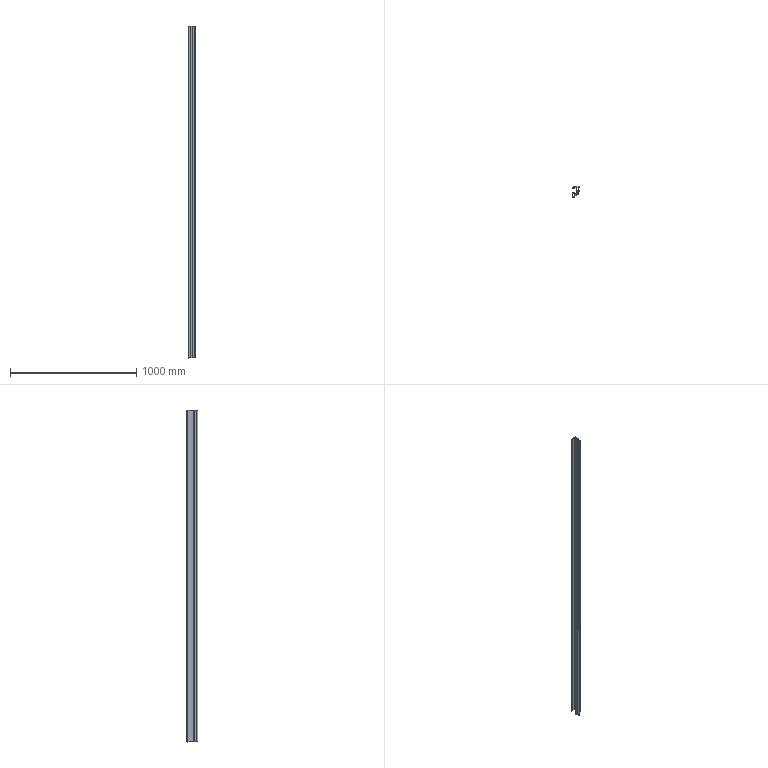Part | STEP file | 51E-01158JG10 | 1 solid | 150 faces | box 62 x 90 x 2631 mm | volume 2262137 mm3 | plane 79 | cylinder 71 | commonest cylinder face diameters 1 x40 0.4 x7 4 x6 6 x5 2 x4 8 x2